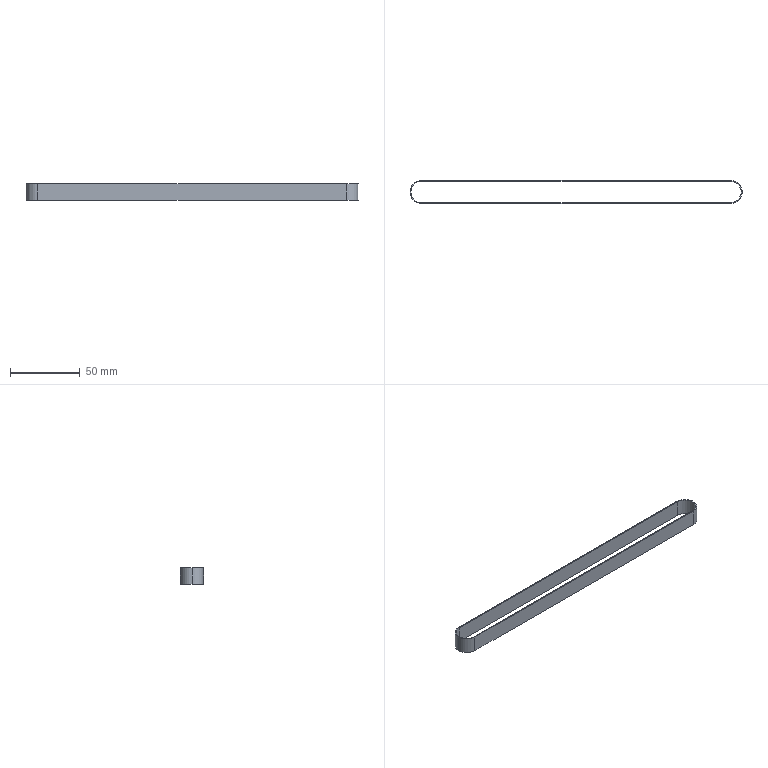Part | SolidWorks | features Extrusion 1 | 1 solid | 12 faces | box 238.67 x 16.67 x 12 mm | volume 3738 mm3 | cylinder 6 | plane 6 | commonest cylinder face diameters 15.41 x3 16.67 x3
STEP:
#1=CARTESIAN_POINT('',(0.,7.705,6.));
#2=VERTEX_POINT('',#1);
#3=CARTESIAN_POINT('',(-7.705,0.,6.));
#4=VERTEX_POINT('',#3);
#5=CARTESIAN_POINT('',(0.,0.,6.));
#6=DIRECTION('',(0.,0.,1.));
#7=DIRECTION('',(1.,0.,0.));
#8=AXIS2_PLACEMENT_3D('',#5,#6,#7);
#9=CIRCLE('',#8,7.705);
#10=EDGE_CURVE('',#2,#4,#9,.T.);
#11=ORIENTED_EDGE('',*,*,#10,.T.);
#12=CARTESIAN_POINT('',(-7.705,0.,-6.));
#13=VERTEX_POINT('',#12);
#14=CARTESIAN_POINT('',(-7.705,0.,6.));
#15=DIRECTION('',(0.,0.,-1.));
#16=VECTOR('',#15,1000.);
#17=LINE('',#14,#16);
#18=EDGE_CURVE('',#4,#13,#17,.T.);
#19=ORIENTED_EDGE('',*,*,#18,.T.);
#20=CARTESIAN_POINT('',(0.,7.705,-6.));
#21=VERTEX_POINT('',#20);
#22=CARTESIAN_POINT('',(0.,0.,-6.));
#23=DIRECTION('',(0.,0.,1.));
#24=DIRECTION('',(1.,0.,0.));
#25=AXIS2_PLACEMENT_3D('',#22,#23,#24);
#26=CIRCLE('',#25,7.705);
#27=EDGE_CURVE('',#21,#13,#26,.T.);
#28=ORIENTED_EDGE('',*,*,#27,.F.);
#29=CARTESIAN_POINT('',(0.,7.705,6.));
#30=DIRECTION('',(0.,0.,-1.));
#31=VECTOR('',#30,1000.);
#32=LINE('',#29,#31);
#33=EDGE_CURVE('',#2,#21,#32,.T.);
#34=ORIENTED_EDGE('',*,*,#33,.F.);
#35=EDGE_LOOP('',(#11,#19,#28,#34));
#36=FACE_OUTER_BOUND('',#35,.T.);
#37=CARTESIAN_POINT('',(0.,0.,6.));
#38=DIRECTION('',(0.,0.,-1.));
#39=DIRECTION('',(-1.,0.,0.));
#40=AXIS2_PLACEMENT_3D('',#37,#38,#39);
#41=CYLINDRICAL_SURFACE('',#40,7.705);
#42=ADVANCED_FACE('',(#36),#41,.F.);
#43=CARTESIAN_POINT('',(-8.335,0.,6.));
#44=VERTEX_POINT('',#43);
#45=CARTESIAN_POINT('',(0.,-8.335,6.));
#46=VERTEX_POINT('',#45);
#47=CARTESIAN_POINT('',(0.,0.,6.));
#48=DIRECTION('',(0.,0.,1.));
#49=DIRECTION('',(1.,0.,0.));
#50=AXIS2_PLACEMENT_3D('',#47,#48,#49);
#51=CIRCLE('',#50,8.335);
#52=EDGE_CURVE('',#44,#46,#51,.T.);
#53=ORIENTED_EDGE('',*,*,#52,.F.);
#54=CARTESIAN_POINT('',(-8.335,0.,-6.));
#55=VERTEX_POINT('',#54);
#56=CARTESIAN_POINT('',(-8.335,0.,6.));
#57=DIRECTION('',(0.,0.,-1.));
#58=VECTOR('',#57,1000.);
#59=LINE('',#56,#58);
#60=EDGE_CURVE('',#44,#55,#59,.T.);
#61=ORIENTED_EDGE('',*,*,#60,.T.);
#62=CARTESIAN_POINT('',(0.,-8.335,-6.));
#63=VERTEX_POINT('',#62);
#64=CARTESIAN_POINT('',(0.,0.,-6.));
#65=DIRECTION('',(0.,0.,1.));
#66=DIRECTION('',(1.,0.,0.));
#67=AXIS2_PLACEMENT_3D('',#64,#65,#66);
#68=CIRCLE('',#67,8.335);
#69=EDGE_CURVE('',#55,#63,#68,.T.);
#70=ORIENTED_EDGE('',*,*,#69,.T.);
#71=CARTESIAN_POINT('',(0.,-8.335,6.));
#72=DIRECTION('',(0.,0.,-1.));
#73=VECTOR('',#72,1000.);
#74=LINE('',#71,#73);
#75=EDGE_CURVE('',#46,#63,#74,.T.);
#76=ORIENTED_EDGE('',*,*,#75,.F.);
#77=EDGE_LOOP('',(#53,#61,#70,#76));
#78=FACE_OUTER_BOUND('',#77,.T.);
#79=CARTESIAN_POINT('',(0.,0.,6.));
#80=DIRECTION('',(0.,0.,-1.));
#81=DIRECTION('',(-1.,0.,0.));
#82=AXIS2_PLACEMENT_3D('',#79,#80,#81);
#83=CYLINDRICAL_SURFACE('',#82,8.335);
#84=ADVANCED_FACE('',(#78),#83,.T.);
#85=CARTESIAN_POINT('',(0.,8.335,6.));
#86=VERTEX_POINT('',#85);
#87=CARTESIAN_POINT('',(0.,0.,6.));
#88=DIRECTION('',(0.,0.,1.));
#89=DIRECTION('',(1.,0.,0.));
#90=AXIS2_PLACEMENT_3D('',#87,#88,#89);
#91=CIRCLE('',#90,8.335);
#92=EDGE_CURVE('',#86,#44,#91,.T.);
#93=ORIENTED_EDGE('',*,*,#92,.T.);
#94=ORIENTED_EDGE('',*,*,#52,.T.);
#95=CARTESIAN_POINT('',(222.,-8.335,6.));
#96=VERTEX_POINT('',#95);
#97=CARTESIAN_POINT('',(222.,-8.335,6.));
#98=DIRECTION('',(1.,0.,0.));
#99=VECTOR('',#98,1000.);
#100=LINE('',#97,#99);
#101=EDGE_CURVE('',#46,#96,#100,.T.);
#102=ORIENTED_EDGE('',*,*,#101,.T.);
#103=CARTESIAN_POINT('',(222.,8.335,6.));
#104=VERTEX_POINT('',#103);
#105=CARTESIAN_POINT('',(222.,0.,6.));
#106=DIRECTION('',(0.,0.,1.));
#107=DIRECTION('',(1.,0.,0.));
#108=AXIS2_PLACEMENT_3D('',#105,#106,#107);
#109=CIRCLE('',#108,8.335);
#110=EDGE_CURVE('',#96,#104,#109,.T.);
#111=ORIENTED_EDGE('',*,*,#110,.T.);
#112=CARTESIAN_POINT('',(0.,8.335,6.));
#113=DIRECTION('',(-1.,0.,0.));
#114=VECTOR('',#113,1000.);
#115=LINE('',#112,#114);
#116=EDGE_CURVE('',#104,#86,#115,.T.);
#117=ORIENTED_EDGE('',*,*,#116,.T.);
#118=EDGE_LOOP('',(#93,#94,#102,#111,#117));
#119=FACE_OUTER_BOUND('',#118,.T.);
#120=CARTESIAN_POINT('',(0.,-7.705,6.));
#121=VERTEX_POINT('',#120);
#122=CARTESIAN_POINT('',(222.,-7.705,6.));
#123=VERTEX_POINT('',#122);
#124=CARTESIAN_POINT('',(222.,-7.705,6.));
#125=DIRECTION('',(1.,0.,0.));
#126=VECTOR('',#125,1000.);
#127=LINE('',#124,#126);
#128=EDGE_CURVE('',#121,#123,#127,.T.);
#129=ORIENTED_EDGE('',*,*,#128,.F.);
#130=CARTESIAN_POINT('',(0.,0.,6.));
#131=DIRECTION('',(0.,0.,1.));
#132=DIRECTION('',(1.,0.,0.));
#133=AXIS2_PLACEMENT_3D('',#130,#131,#132);
#134=CIRCLE('',#133,7.705);
#135=EDGE_CURVE('',#4,#121,#134,.T.);
#136=ORIENTED_EDGE('',*,*,#135,.F.);
#137=ORIENTED_EDGE('',*,*,#10,.F.);
#138=CARTESIAN_POINT('',(222.,7.705,6.));
#139=VERTEX_POINT('',#138);
#140=CARTESIAN_POINT('',(0.,7.705,6.));
#141=DIRECTION('',(-1.,0.,0.));
#142=VECTOR('',#141,1000.);
#143=LINE('',#140,#142);
#144=EDGE_CURVE('',#139,#2,#143,.T.);
#145=ORIENTED_EDGE('',*,*,#144,.F.);
#146=CARTESIAN_POINT('',(222.,0.,6.));
#147=DIRECTION('',(0.,0.,1.));
#148=DIRECTION('',(1.,0.,0.));
#149=AXIS2_PLACEMENT_3D('',#146,#147,#148);
#150=CIRCLE('',#149,7.705);
#151=EDGE_CURVE('',#123,#139,#150,.T.);
#152=ORIENTED_EDGE('',*,*,#151,.F.);
#153=EDGE_LOOP('',(#129,#136,#137,#145,#152));
#154=FACE_BOUND('',#153,.T.);
#155=CARTESIAN_POINT('',(0.,0.,6.));
#156=DIRECTION('',(0.,0.,1.));
#157=DIRECTION('',(1.,0.,0.));
#158=AXIS2_PLACEMENT_3D('',#155,#156,#157);
#159=PLANE('',#158);
#160=ADVANCED_FACE('',(#119,#154),#159,.T.);
#161=CARTESIAN_POINT('',(0.,8.335,-6.));
#162=VERTEX_POINT('',#161);
#163=CARTESIAN_POINT('',(0.,0.,-6.));
#164=DIRECTION('',(0.,0.,1.));
#165=DIRECTION('',(1.,0.,0.));
#166=AXIS2_PLACEMENT_3D('',#163,#164,#165);
#167=CIRCLE('',#166,8.335);
#168=EDGE_CURVE('',#162,#55,#167,.T.);
#169=ORIENTED_EDGE('',*,*,#168,.F.);
#170=CARTESIAN_POINT('',(222.,8.335,-6.));
#171=VERTEX_POINT('',#170);
#172=CARTESIAN_POINT('',(0.,8.335,-6.));
#173=DIRECTION('',(-1.,0.,0.));
#174=VECTOR('',#173,1000.);
#175=LINE('',#172,#174);
#176=EDGE_CURVE('',#171,#162,#175,.T.);
#177=ORIENTED_EDGE('',*,*,#176,.F.);
#178=CARTESIAN_POINT('',(222.,-8.335,-6.));
#179=VERTEX_POINT('',#178);
#180=CARTESIAN_POINT('',(222.,0.,-6.));
#181=DIRECTION('',(0.,0.,1.));
#182=DIRECTION('',(1.,0.,0.));
#183=AXIS2_PLACEMENT_3D('',#180,#181,#182);
#184=CIRCLE('',#183,8.335);
#185=EDGE_CURVE('',#179,#171,#184,.T.);
#186=ORIENTED_EDGE('',*,*,#185,.F.);
#187=CARTESIAN_POINT('',(222.,-8.335,-6.));
#188=DIRECTION('',(1.,0.,0.));
#189=VECTOR('',#188,1000.);
#190=LINE('',#187,#189);
#191=EDGE_CURVE('',#63,#179,#190,.T.);
#192=ORIENTED_EDGE('',*,*,#191,.F.);
#193=ORIENTED_EDGE('',*,*,#69,.F.);
#194=EDGE_LOOP('',(#169,#177,#186,#192,#193));
#195=FACE_OUTER_BOUND('',#194,.T.);
#196=ORIENTED_EDGE('',*,*,#27,.T.);
#197=CARTESIAN_POINT('',(0.,-7.705,-6.));
#198=VERTEX_POINT('',#197);
#199=CARTESIAN_POINT('',(0.,0.,-6.));
#200=DIRECTION('',(0.,0.,1.));
#201=DIRECTION('',(1.,0.,0.));
#202=AXIS2_PLACEMENT_3D('',#199,#200,#201);
#203=CIRCLE('',#202,7.705);
#204=EDGE_CURVE('',#13,#198,#203,.T.);
#205=ORIENTED_EDGE('',*,*,#204,.T.);
#206=CARTESIAN_POINT('',(222.,-7.705,-6.));
#207=VERTEX_POINT('',#206);
#208=CARTESIAN_POINT('',(222.,-7.705,-6.));
#209=DIRECTION('',(1.,0.,0.));
#210=VECTOR('',#209,1000.);
#211=LINE('',#208,#210);
#212=EDGE_CURVE('',#198,#207,#211,.T.);
#213=ORIENTED_EDGE('',*,*,#212,.T.);
#214=CARTESIAN_POINT('',(222.,7.705,-6.));
#215=VERTEX_POINT('',#214);
#216=CARTESIAN_POINT('',(222.,0.,-6.));
#217=DIRECTION('',(0.,0.,1.));
#218=DIRECTION('',(1.,0.,0.));
#219=AXIS2_PLACEMENT_3D('',#216,#217,#218);
#220=CIRCLE('',#219,7.705);
#221=EDGE_CURVE('',#207,#215,#220,.T.);
#222=ORIENTED_EDGE('',*,*,#221,.T.);
#223=CARTESIAN_POINT('',(0.,7.705,-6.));
#224=DIRECTION('',(-1.,0.,0.));
#225=VECTOR('',#224,1000.);
#226=LINE('',#223,#225);
#227=EDGE_CURVE('',#215,#21,#226,.T.);
#228=ORIENTED_EDGE('',*,*,#227,.T.);
#229=EDGE_LOOP('',(#196,#205,#213,#222,#228));
#230=FACE_BOUND('',#229,.T.);
#231=CARTESIAN_POINT('',(0.,0.,-6.));
#232=DIRECTION('',(0.,0.,1.));
#233=DIRECTION('',(1.,0.,0.));
#234=AXIS2_PLACEMENT_3D('',#231,#232,#233);
#235=PLANE('',#234);
#236=ADVANCED_FACE('',(#195,#230),#235,.F.);
#237=ORIENTED_EDGE('',*,*,#60,.F.);
#238=ORIENTED_EDGE('',*,*,#92,.F.);
#239=CARTESIAN_POINT('',(0.,8.335,6.));
#240=DIRECTION('',(0.,0.,-1.));
#241=VECTOR('',#240,1000.);
#242=LINE('',#239,#241);
#243=EDGE_CURVE('',#86,#162,#242,.T.);
#244=ORIENTED_EDGE('',*,*,#243,.T.);
#245=ORIENTED_EDGE('',*,*,#168,.T.);
#246=EDGE_LOOP('',(#237,#238,#244,#245));
#247=FACE_OUTER_BOUND('',#246,.T.);
#248=CARTESIAN_POINT('',(0.,0.,6.));
#249=DIRECTION('',(0.,0.,-1.));
#250=DIRECTION('',(-1.,0.,0.));
#251=AXIS2_PLACEMENT_3D('',#248,#249,#250);
#252=CYLINDRICAL_SURFACE('',#251,8.335);
#253=ADVANCED_FACE('',(#247),#252,.T.);
#254=ORIENTED_EDGE('',*,*,#191,.T.);
#255=CARTESIAN_POINT('',(222.,-8.335,6.));
#256=DIRECTION('',(0.,0.,-1.));
#257=VECTOR('',#256,1000.);
#258=LINE('',#255,#257);
#259=EDGE_CURVE('',#96,#179,#258,.T.);
#260=ORIENTED_EDGE('',*,*,#259,.F.);
#261=ORIENTED_EDGE('',*,*,#101,.F.);
#262=ORIENTED_EDGE('',*,*,#75,.T.);
#263=EDGE_LOOP('',(#254,#260,#261,#262));
#264=FACE_OUTER_BOUND('',#263,.T.);
#265=CARTESIAN_POINT('',(222.,-8.335,6.));
#266=DIRECTION('',(0.,1.,0.));
#267=DIRECTION('',(0.,0.,1.));
#268=AXIS2_PLACEMENT_3D('',#265,#266,#267);
#269=PLANE('',#268);
#270=ADVANCED_FACE('',(#264),#269,.F.);
#271=ORIENTED_EDGE('',*,*,#185,.T.);
#272=CARTESIAN_POINT('',(222.,8.335,6.));
#273=DIRECTION('',(0.,0.,-1.));
#274=VECTOR('',#273,1000.);
#275=LINE('',#272,#274);
#276=EDGE_CURVE('',#104,#171,#275,.T.);
#277=ORIENTED_EDGE('',*,*,#276,.F.);
#278=ORIENTED_EDGE('',*,*,#110,.F.);
#279=ORIENTED_EDGE('',*,*,#259,.T.);
#280=EDGE_LOOP('',(#271,#277,#278,#279));
#281=FACE_OUTER_BOUND('',#280,.T.);
#282=CARTESIAN_POINT('',(222.,0.,6.));
#283=DIRECTION('',(0.,0.,-1.));
#284=DIRECTION('',(-1.,0.,0.));
#285=AXIS2_PLACEMENT_3D('',#282,#283,#284);
#286=CYLINDRICAL_SURFACE('',#285,8.335);
#287=ADVANCED_FACE('',(#281),#286,.T.);
#288=ORIENTED_EDGE('',*,*,#176,.T.);
#289=ORIENTED_EDGE('',*,*,#243,.F.);
#290=ORIENTED_EDGE('',*,*,#116,.F.);
#291=ORIENTED_EDGE('',*,*,#276,.T.);
#292=EDGE_LOOP('',(#288,#289,#290,#291));
#293=FACE_OUTER_BOUND('',#292,.T.);
#294=CARTESIAN_POINT('',(0.,8.335,6.));
#295=DIRECTION('',(0.,-1.,0.));
#296=DIRECTION('',(0.,0.,-1.));
#297=AXIS2_PLACEMENT_3D('',#294,#295,#296);
#298=PLANE('',#297);
#299=ADVANCED_FACE('',(#293),#298,.F.);
#300=ORIENTED_EDGE('',*,*,#18,.F.);
#301=ORIENTED_EDGE('',*,*,#135,.T.);
#302=CARTESIAN_POINT('',(0.,-7.705,6.));
#303=DIRECTION('',(0.,0.,-1.));
#304=VECTOR('',#303,1000.);
#305=LINE('',#302,#304);
#306=EDGE_CURVE('',#121,#198,#305,.T.);
#307=ORIENTED_EDGE('',*,*,#306,.T.);
#308=ORIENTED_EDGE('',*,*,#204,.F.);
#309=EDGE_LOOP('',(#300,#301,#307,#308));
#310=FACE_OUTER_BOUND('',#309,.T.);
#311=CARTESIAN_POINT('',(0.,0.,6.));
#312=DIRECTION('',(0.,0.,-1.));
#313=DIRECTION('',(-1.,0.,0.));
#314=AXIS2_PLACEMENT_3D('',#311,#312,#313);
#315=CYLINDRICAL_SURFACE('',#314,7.705);
#316=ADVANCED_FACE('',(#310),#315,.F.);
#317=ORIENTED_EDGE('',*,*,#212,.F.);
#318=ORIENTED_EDGE('',*,*,#306,.F.);
#319=ORIENTED_EDGE('',*,*,#128,.T.);
#320=CARTESIAN_POINT('',(222.,-7.705,6.));
#321=DIRECTION('',(0.,0.,-1.));
#322=VECTOR('',#321,1000.);
#323=LINE('',#320,#322);
#324=EDGE_CURVE('',#123,#207,#323,.T.);
#325=ORIENTED_EDGE('',*,*,#324,.T.);
#326=EDGE_LOOP('',(#317,#318,#319,#325));
#327=FACE_OUTER_BOUND('',#326,.T.);
#328=CARTESIAN_POINT('',(222.,-7.705,6.));
#329=DIRECTION('',(0.,1.,0.));
#330=DIRECTION('',(0.,0.,1.));
#331=AXIS2_PLACEMENT_3D('',#328,#329,#330);
#332=PLANE('',#331);
#333=ADVANCED_FACE('',(#327),#332,.T.);
#334=ORIENTED_EDGE('',*,*,#221,.F.);
#335=ORIENTED_EDGE('',*,*,#324,.F.);
#336=ORIENTED_EDGE('',*,*,#151,.T.);
#337=CARTESIAN_POINT('',(222.,7.705,6.));
#338=DIRECTION('',(0.,0.,-1.));
#339=VECTOR('',#338,1000.);
#340=LINE('',#337,#339);
#341=EDGE_CURVE('',#139,#215,#340,.T.);
#342=ORIENTED_EDGE('',*,*,#341,.T.);
#343=EDGE_LOOP('',(#334,#335,#336,#342));
#344=FACE_OUTER_BOUND('',#343,.T.);
#345=CARTESIAN_POINT('',(222.,0.,6.));
#346=DIRECTION('',(0.,0.,-1.));
#347=DIRECTION('',(-1.,0.,0.));
#348=AXIS2_PLACEMENT_3D('',#345,#346,#347);
#349=CYLINDRICAL_SURFACE('',#348,7.705);
#350=ADVANCED_FACE('',(#344),#349,.F.);
#351=ORIENTED_EDGE('',*,*,#227,.F.);
#352=ORIENTED_EDGE('',*,*,#341,.F.);
#353=ORIENTED_EDGE('',*,*,#144,.T.);
#354=ORIENTED_EDGE('',*,*,#33,.T.);
#355=EDGE_LOOP('',(#351,#352,#353,#354));
#356=FACE_OUTER_BOUND('',#355,.T.);
#357=CARTESIAN_POINT('',(0.,7.705,6.));
#358=DIRECTION('',(0.,-1.,0.));
#359=DIRECTION('',(0.,0.,-1.));
#360=AXIS2_PLACEMENT_3D('',#357,#358,#359);
#361=PLANE('',#360);
#362=ADVANCED_FACE('',(#356),#361,.T.);
#363=CLOSED_SHELL('',(#42,#84,#160,#236,#253,#270,#287,#299,#316,#333,#350,#362));
#364=MANIFOLD_SOLID_BREP('',#363);
#365=CARTESIAN_POINT('',(0.,0.,0.));
#366=DIRECTION('',(0.,0.,1.));
#367=DIRECTION('',(1.,0.,0.));
#368=AXIS2_PLACEMENT_3D('',#365,#366,#367);
#369=(LENGTH_UNIT()NAMED_UNIT(*)SI_UNIT(.MILLI.,.METRE.));
#370=UNCERTAINTY_MEASURE_WITH_UNIT(LENGTH_MEASURE(0.00001),#369,'','');
#371=(NAMED_UNIT(*)PLANE_ANGLE_UNIT()SI_UNIT($,.RADIAN.));
#372=(NAMED_UNIT(*)SI_UNIT($,.STERADIAN.)SOLID_ANGLE_UNIT());
#373=(GEOMETRIC_REPRESENTATION_CONTEXT(3)GLOBAL_UNCERTAINTY_ASSIGNED_CONTEXT((#370))GLOBAL_UNIT_ASSIGNED_CONTEXT((#369,#371,#372))REPRESENTATION_CONTEXT('',''));
#374=ADVANCED_BREP_SHAPE_REPRESENTATION('',(#364,#368),#373);